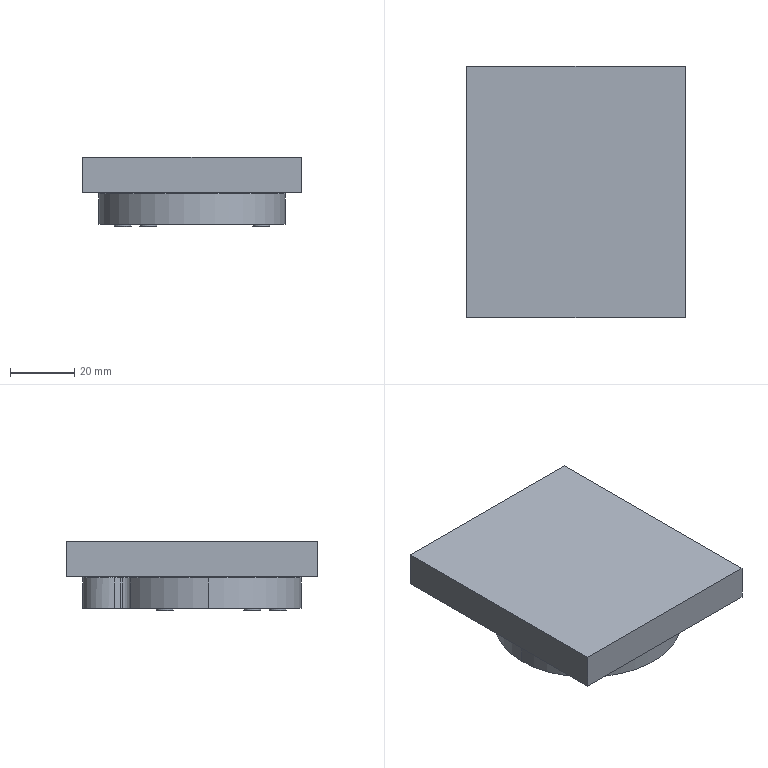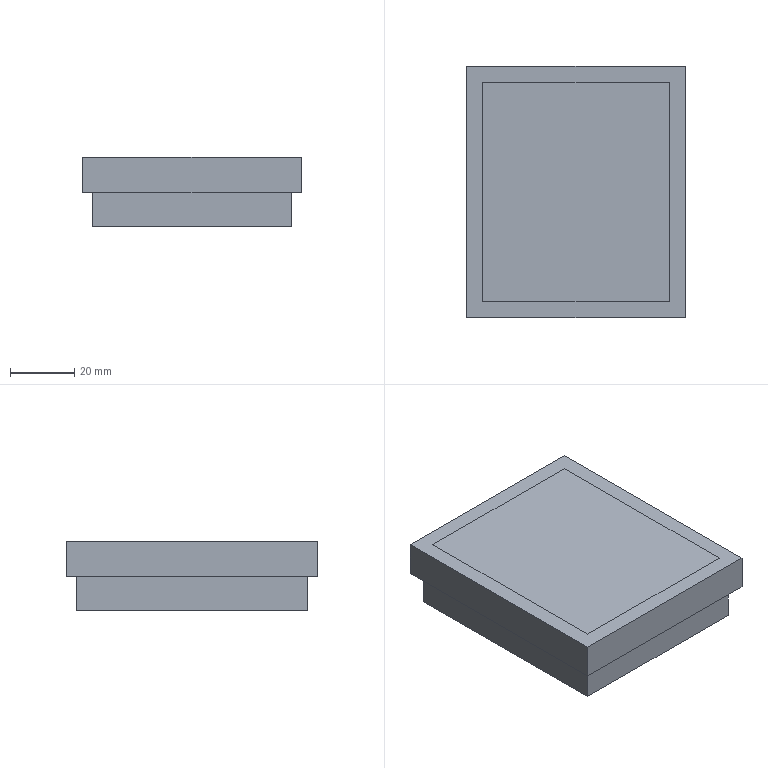CAM job | NX | 3-axis milling, drilling | part box 68 x 78.27 x 21.8 mm | stock box 68 x 78.27 x 21.8 mm
Tools:
number,name,description,diameter,corner_radius,flute_length,length,flutes
19,D80,Milling Tool-5 Parameters,80.0,0.0,50.0,75.0,2
15,D10,Milling Tool-5 Parameters,10.0,0.0,50.0,75.0,2
11,D4,Milling Tool-5 Parameters,4.0,0.0,50.0,75.0,2
1,D6A45,Milling Tool-5 Parameters,6.0,0.0,50.0,75.0,2
16,1.6ZT,Drilling Tool,1.6,0.0,35.0,50.0,2
7,3.5ZT,Drilling Tool,3.5,0.0,35.0,50.0,2
17,D2,Milling Tool-5 Parameters,2.0,0.0,50.0,75.0,2
18,D3R0.5,Milling Tool-5 Parameters,3.0,0.5,50.0,75.0,2
Operations:
program,operation,operation_type,tool,method,geometry_group,spindle_rpm,surface_speed,feed_per_tooth,feed_cut,feed_plunge,cut_length_mm,path_length_mm,cut_time_min,machine_time_min
1,FLOOR_WALL,VolumeBased25DMillingOperation,D80,METHOD,A,5000.0,1256.0,0.12,1200.0,100.0,154.0,208.0,0.1283,0.1337
1,CAVITY_MILL,CavityMilling,D10,METHOD,A,9500.0,298.0,0.1842,3500.0,1000.0,13009.043,13454.578,3.83,3.875
1,FLOOR_WALL_1,VolumeBased25DMillingOperation,D10,METHOD,A,9500.0,298.0,0.0658,1250.0,1000.0,1165.914,1316.988,0.9369,0.952
1,ZLEVEL_PROFILE_1,ZLevelMilling,D4,METHOD,A,9500.0,119.0,0.1316,2500.0,1000.0,717.283,782.283,0.3087,0.3152
1,ZLEVEL_PROFILE_1_COPY,ZLevelMilling,D4,METHOD,A,9500.0,119.0,0.1053,2000.0,1000.0,401.563,895.727,0.2497,0.2991
1,ZLEVEL_PROFILE,ZLevelMilling,D4,METHOD,A,9500.0,119.0,0.0632,1200.0,1000.0,195.41,262.41,0.1676,0.1743
1,ZLEVEL_PROFILE_COPY,ZLevelMilling,D4,METHOD,A,9500.0,119.0,0.0632,1200.0,1000.0,240.802,331.402,0.2054,0.2145
1,SPOT_DRILLING,Operation,D6A45,METHOD,A,9500.0,179.0,0.0132,250.0,0.0,20.0,220.167,0.08,0.1
1,DRILLING_COPY_COPY_COPY,Operation,1.6ZT,METHOD,A,2500.0,12.0,0.016,80.0,0.0,25.961,131.202,0.3245,0.335
1,DRILLING_COPY_COPY_COPY_1,Operation,3.5ZT,METHOD,A,2500.0,19.0,0.02,100.0,0.0,49.054,248.483,0.4905,0.5105
1,HOLE_MILLING_2,CylinderMilling,D4,METHOD,A,9500.0,119.0,0.0658,1250.0,100.0,382.419,690.044,0.3059,0.3367
1,PLANAR_PROFILE,PlanarMilling,D6A45,METHOD,A,9500.0,179.0,0.0789,1500.0,500.0,265.751,630.954,0.2004,0.2369
1,PLANAR_PROFILE_COPY,PlanarMilling,D6A45,METHOD,A,9500.0,179.0,0.0789,1500.0,500.0,120.168,246.26,0.0879,0.1005
2,FLOOR_WALL_COPY,VolumeBased25DMillingOperation,D80,METHOD,B,5000.0,1256.0,0.2,2000.0,100.0,750.0,1575.401,0.375,0.4575
2,FLOOR_WALL_COPY_1,VolumeBased25DMillingOperation,D80,METHOD,B,5000.0,1256.0,0.12,1200.0,100.0,150.0,204.0,0.125,0.1304
2,CAVITY_MILL_COPY,CavityMilling,D10,METHOD,B,9500.0,298.0,0.1842,3500.0,1000.0,3916.308,4170.82,1.433,1.458
2,CAVITY_MILL_COPY_COPY,CavityMilling,D4,METHOD,B,9500.0,119.0,0.1053,2000.0,1000.0,1478.9,2928.525,0.9112,1.056
2,FLOOR_WALL_2,VolumeBased25DMillingOperation,D4,METHOD,B,9500.0,119.0,0.0658,1250.0,100.0,1371.384,1806.294,1.097,1.141
2,FLOOR_WALL_2_COPY,VolumeBased25DMillingOperation,D4,METHOD,B,9500.0,119.0,0.0658,1250.0,100.0,865.832,1225.258,0.6927,0.7286
2,CAVITY_MILL_COPY_COPY_COPY,CavityMilling,D2,METHOD,B,9500.0,119.0,0.1053,2000.0,1000.0,387.688,785.427,0.2585,0.2983
2,ZLEVEL_PROFILE_1_1,ZLevelMilling,D3R0.5,METHOD,B,9500.0,89.0,0.1316,2500.0,1000.0,2110.841,2491.326,0.8499,0.8879
2,PLANAR_MILL,PlanarMilling,D6A45,METHOD,B,9500.0,179.0,0.0658,1250.0,100.0,408.896,537.054,0.3271,0.3399
2,PLANAR_MILL_COPY,PlanarMilling,D6A45,METHOD,B,9500.0,179.0,0.0658,1250.0,100.0,27.221,277.01,0.0218,0.0468
3,FLOOR_WALL_3,VolumeBased25DMillingOperation,D4,METHOD,C,9500.0,119.0,0.1316,2500.0,1000.0,20381.353,20881.151,8.393,8.443
3,FLOOR_WALL_3_COPY,VolumeBased25DMillingOperation,D4,METHOD,C,9500.0,119.0,0.0789,1500.0,1000.0,190.394,260.394,0.1277,0.1347